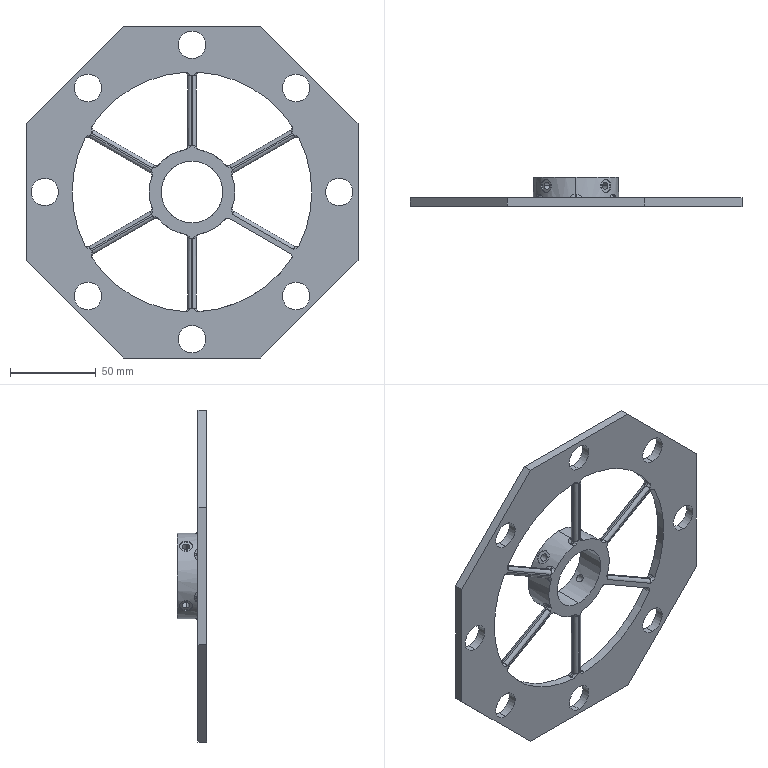Part | SolidWorks | features ICE 5, CirPattern 3, Fillet 2, Extrusion 1 | 1 solid | 175 faces | volume 92425 mm3 | cylinder 95 | spline 46 | plane 27 | torus 7 | commonest cylinder face diameters 4 x53 16 x16 4.4 x8 8 x8 140 x6 36 x2